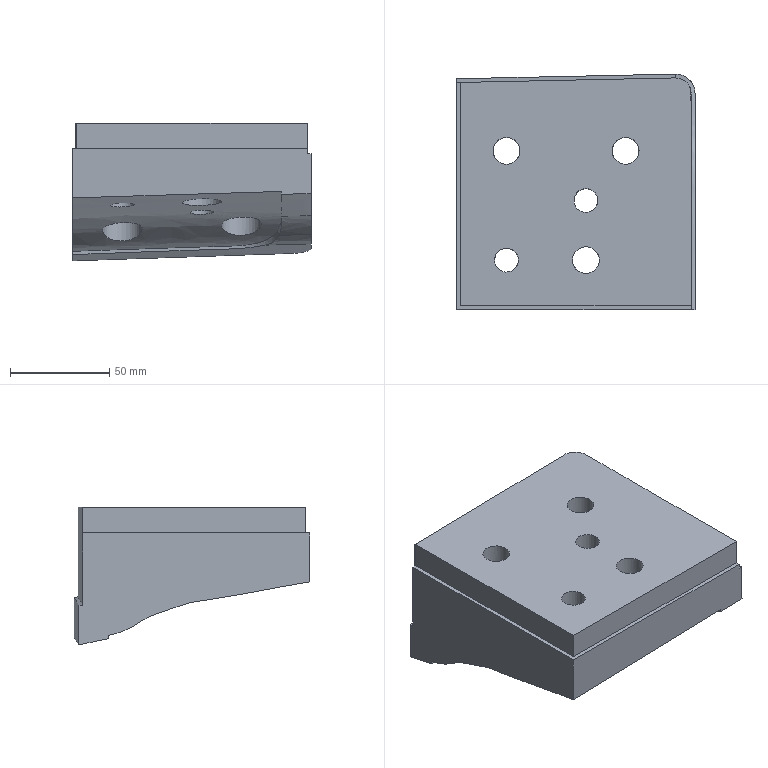Part | NX | features solid 2 | 1 solid | 30 faces | box 120.032 x 118.765 x 69.362 mm | volume 617625 mm3 | spline 12 | plane 10 | cylinder 8 | commonest cylinder face diameters 13.5 x3 20 x3 12 x2